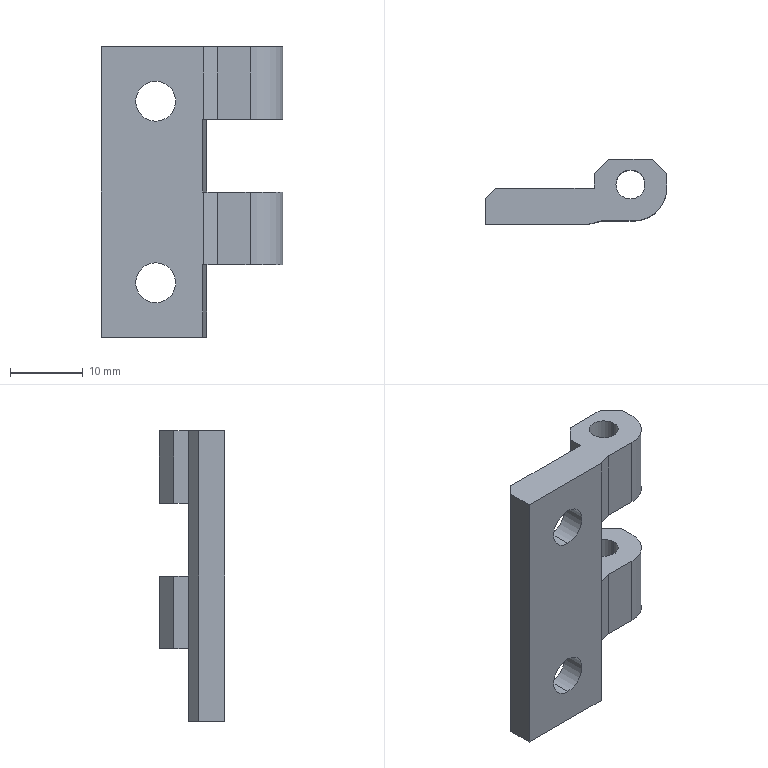Part | SolidWorks | features BaseBody 1 | 1 solid | 41 faces | box 25 x 9 x 40 mm | volume 3717 mm3 | plane 27 | cylinder 14 | commonest cylinder face diameters 4 x4 5.5 x4 10.5 x4 9 x2
STEP:
#1=CARTESIAN_POINT('',(-12.5,3.3,15.25));
#2=VERTEX_POINT('',#1);
#3=CARTESIAN_POINT('',(-12.5,3.3,9.75));
#4=VERTEX_POINT('',#3);
#5=CARTESIAN_POINT('',(-12.5,3.3,12.5));
#6=DIRECTION('',(0.,-1.,0.));
#7=DIRECTION('',(0.,0.,-1.));
#8=AXIS2_PLACEMENT_3D('',#5,#6,#7);
#9=CIRCLE('',#8,2.75);
#10=EDGE_CURVE('',#2,#4,#9,.T.);
#11=ORIENTED_EDGE('',*,*,#10,.F.);
#12=CARTESIAN_POINT('',(-12.5,0.,15.25));
#13=VERTEX_POINT('',#12);
#14=CARTESIAN_POINT('',(-12.5,0.,15.25));
#15=DIRECTION('',(0.,-1.,0.));
#16=VECTOR('',#15,1000.);
#17=LINE('',#14,#16);
#18=EDGE_CURVE('',#2,#13,#17,.T.);
#19=ORIENTED_EDGE('',*,*,#18,.T.);
#20=CARTESIAN_POINT('',(-12.5,0.,9.75));
#21=VERTEX_POINT('',#20);
#22=CARTESIAN_POINT('',(-12.5,0.,12.5));
#23=DIRECTION('',(0.,-1.,0.));
#24=DIRECTION('',(0.,0.,-1.));
#25=AXIS2_PLACEMENT_3D('',#22,#23,#24);
#26=CIRCLE('',#25,2.75);
#27=EDGE_CURVE('',#13,#21,#26,.T.);
#28=ORIENTED_EDGE('',*,*,#27,.T.);
#29=CARTESIAN_POINT('',(-12.5,0.,9.75));
#30=DIRECTION('',(0.,-1.,0.));
#31=VECTOR('',#30,1000.);
#32=LINE('',#29,#31);
#33=EDGE_CURVE('',#4,#21,#32,.T.);
#34=ORIENTED_EDGE('',*,*,#33,.F.);
#35=EDGE_LOOP('',(#11,#19,#28,#34));
#36=FACE_OUTER_BOUND('',#35,.T.);
#37=CARTESIAN_POINT('',(-12.5,0.,12.5));
#38=DIRECTION('',(0.,-1.,0.));
#39=DIRECTION('',(0.,0.,-1.));
#40=AXIS2_PLACEMENT_3D('',#37,#38,#39);
#41=CYLINDRICAL_SURFACE('',#40,2.75);
#42=ADVANCED_FACE('',(#36),#41,.F.);
#43=CARTESIAN_POINT('',(-12.5,3.3,-9.75));
#44=VERTEX_POINT('',#43);
#45=CARTESIAN_POINT('',(-12.5,3.3,-15.25));
#46=VERTEX_POINT('',#45);
#47=CARTESIAN_POINT('',(-12.5,3.3,-12.5));
#48=DIRECTION('',(0.,-1.,0.));
#49=DIRECTION('',(0.,0.,-1.));
#50=AXIS2_PLACEMENT_3D('',#47,#48,#49);
#51=CIRCLE('',#50,2.75);
#52=EDGE_CURVE('',#44,#46,#51,.T.);
#53=ORIENTED_EDGE('',*,*,#52,.F.);
#54=CARTESIAN_POINT('',(-12.5,0.,-9.75));
#55=VERTEX_POINT('',#54);
#56=CARTESIAN_POINT('',(-12.5,0.,-9.75));
#57=DIRECTION('',(0.,-1.,0.));
#58=VECTOR('',#57,1000.);
#59=LINE('',#56,#58);
#60=EDGE_CURVE('',#44,#55,#59,.T.);
#61=ORIENTED_EDGE('',*,*,#60,.T.);
#62=CARTESIAN_POINT('',(-12.5,0.,-15.25));
#63=VERTEX_POINT('',#62);
#64=CARTESIAN_POINT('',(-12.5,0.,-12.5));
#65=DIRECTION('',(0.,-1.,0.));
#66=DIRECTION('',(0.,0.,-1.));
#67=AXIS2_PLACEMENT_3D('',#64,#65,#66);
#68=CIRCLE('',#67,2.75);
#69=EDGE_CURVE('',#55,#63,#68,.T.);
#70=ORIENTED_EDGE('',*,*,#69,.T.);
#71=CARTESIAN_POINT('',(-12.5,0.,-15.25));
#72=DIRECTION('',(0.,-1.,0.));
#73=VECTOR('',#72,1000.);
#74=LINE('',#71,#73);
#75=EDGE_CURVE('',#46,#63,#74,.T.);
#76=ORIENTED_EDGE('',*,*,#75,.F.);
#77=EDGE_LOOP('',(#53,#61,#70,#76));
#78=FACE_OUTER_BOUND('',#77,.T.);
#79=CARTESIAN_POINT('',(-12.5,0.,-12.5));
#80=DIRECTION('',(0.,-1.,0.));
#81=DIRECTION('',(0.,0.,-1.));
#82=AXIS2_PLACEMENT_3D('',#79,#80,#81);
#83=CYLINDRICAL_SURFACE('',#82,2.75);
#84=ADVANCED_FACE('',(#78),#83,.F.);
#85=CARTESIAN_POINT('',(2.,5.5,20.));
#86=VERTEX_POINT('',#85);
#87=CARTESIAN_POINT('',(-2.,5.5,20.));
#88=VERTEX_POINT('',#87);
#89=CARTESIAN_POINT('',(0.,5.5,20.));
#90=DIRECTION('',(0.,0.,-1.));
#91=DIRECTION('',(-1.,0.,0.));
#92=AXIS2_PLACEMENT_3D('',#89,#90,#91);
#93=CIRCLE('',#92,2.);
#94=EDGE_CURVE('',#86,#88,#93,.T.);
#95=ORIENTED_EDGE('',*,*,#94,.F.);
#96=CARTESIAN_POINT('',(2.,5.5,10.));
#97=VERTEX_POINT('',#96);
#98=CARTESIAN_POINT('',(2.,5.5,20.));
#99=DIRECTION('',(0.,0.,-1.));
#100=VECTOR('',#99,1000.);
#101=LINE('',#98,#100);
#102=EDGE_CURVE('',#86,#97,#101,.T.);
#103=ORIENTED_EDGE('',*,*,#102,.T.);
#104=CARTESIAN_POINT('',(-2.,5.5,10.));
#105=VERTEX_POINT('',#104);
#106=CARTESIAN_POINT('',(0.,5.5,10.));
#107=DIRECTION('',(0.,0.,-1.));
#108=DIRECTION('',(-1.,0.,0.));
#109=AXIS2_PLACEMENT_3D('',#106,#107,#108);
#110=CIRCLE('',#109,2.);
#111=EDGE_CURVE('',#97,#105,#110,.T.);
#112=ORIENTED_EDGE('',*,*,#111,.T.);
#113=CARTESIAN_POINT('',(-2.,5.5,20.));
#114=DIRECTION('',(0.,0.,-1.));
#115=VECTOR('',#114,1000.);
#116=LINE('',#113,#115);
#117=EDGE_CURVE('',#88,#105,#116,.T.);
#118=ORIENTED_EDGE('',*,*,#117,.F.);
#119=EDGE_LOOP('',(#95,#103,#112,#118));
#120=FACE_OUTER_BOUND('',#119,.T.);
#121=CARTESIAN_POINT('',(0.,5.5,20.));
#122=DIRECTION('',(0.,0.,-1.));
#123=DIRECTION('',(-1.,0.,0.));
#124=AXIS2_PLACEMENT_3D('',#121,#122,#123);
#125=CYLINDRICAL_SURFACE('',#124,2.);
#126=ADVANCED_FACE('',(#120),#125,.F.);
#127=CARTESIAN_POINT('',(-12.5,5.,7.25));
#128=VERTEX_POINT('',#127);
#129=CARTESIAN_POINT('',(-12.5,5.,17.75));
#130=VERTEX_POINT('',#129);
#131=CARTESIAN_POINT('',(-12.5,5.,12.5));
#132=DIRECTION('',(0.,1.,0.));
#133=DIRECTION('',(0.,0.,-1.));
#134=AXIS2_PLACEMENT_3D('',#131,#132,#133);
#135=CIRCLE('',#134,5.25);
#136=EDGE_CURVE('',#128,#130,#135,.T.);
#137=ORIENTED_EDGE('',*,*,#136,.T.);
#138=CARTESIAN_POINT('',(-12.5,3.3,17.75));
#139=VERTEX_POINT('',#138);
#140=CARTESIAN_POINT('',(-12.5,0.,17.75));
#141=DIRECTION('',(0.,-1.,0.));
#142=VECTOR('',#141,1000.);
#143=LINE('',#140,#142);
#144=EDGE_CURVE('',#130,#139,#143,.T.);
#145=ORIENTED_EDGE('',*,*,#144,.T.);
#146=CARTESIAN_POINT('',(-12.5,3.3,7.25));
#147=VERTEX_POINT('',#146);
#148=CARTESIAN_POINT('',(-12.5,3.3,12.5));
#149=DIRECTION('',(0.,1.,0.));
#150=DIRECTION('',(0.,0.,-1.));
#151=AXIS2_PLACEMENT_3D('',#148,#149,#150);
#152=CIRCLE('',#151,5.25);
#153=EDGE_CURVE('',#147,#139,#152,.T.);
#154=ORIENTED_EDGE('',*,*,#153,.F.);
#155=CARTESIAN_POINT('',(-12.5,0.,7.25));
#156=DIRECTION('',(0.,-1.,0.));
#157=VECTOR('',#156,1000.);
#158=LINE('',#155,#157);
#159=EDGE_CURVE('',#128,#147,#158,.T.);
#160=ORIENTED_EDGE('',*,*,#159,.F.);
#161=EDGE_LOOP('',(#137,#145,#154,#160));
#162=FACE_OUTER_BOUND('',#161,.T.);
#163=CARTESIAN_POINT('',(-12.5,0.,12.5));
#164=DIRECTION('',(0.,-1.,0.));
#165=DIRECTION('',(0.,0.,-1.));
#166=AXIS2_PLACEMENT_3D('',#163,#164,#165);
#167=CYLINDRICAL_SURFACE('',#166,5.25);
#168=ADVANCED_FACE('',(#162),#167,.F.);
#169=CARTESIAN_POINT('',(-12.5,5.,-17.75));
#170=VERTEX_POINT('',#169);
#171=CARTESIAN_POINT('',(-12.5,5.,-7.25));
#172=VERTEX_POINT('',#171);
#173=CARTESIAN_POINT('',(-12.5,5.,-12.5));
#174=DIRECTION('',(0.,1.,0.));
#175=DIRECTION('',(0.,0.,-1.));
#176=AXIS2_PLACEMENT_3D('',#173,#174,#175);
#177=CIRCLE('',#176,5.25);
#178=EDGE_CURVE('',#170,#172,#177,.T.);
#179=ORIENTED_EDGE('',*,*,#178,.T.);
#180=CARTESIAN_POINT('',(-12.5,3.3,-7.25));
#181=VERTEX_POINT('',#180);
#182=CARTESIAN_POINT('',(-12.5,0.,-7.25));
#183=DIRECTION('',(0.,-1.,0.));
#184=VECTOR('',#183,1000.);
#185=LINE('',#182,#184);
#186=EDGE_CURVE('',#172,#181,#185,.T.);
#187=ORIENTED_EDGE('',*,*,#186,.T.);
#188=CARTESIAN_POINT('',(-12.5,3.3,-17.75));
#189=VERTEX_POINT('',#188);
#190=CARTESIAN_POINT('',(-12.5,3.3,-12.5));
#191=DIRECTION('',(0.,1.,0.));
#192=DIRECTION('',(0.,0.,-1.));
#193=AXIS2_PLACEMENT_3D('',#190,#191,#192);
#194=CIRCLE('',#193,5.25);
#195=EDGE_CURVE('',#189,#181,#194,.T.);
#196=ORIENTED_EDGE('',*,*,#195,.F.);
#197=CARTESIAN_POINT('',(-12.5,0.,-17.75));
#198=DIRECTION('',(0.,-1.,0.));
#199=VECTOR('',#198,1000.);
#200=LINE('',#197,#199);
#201=EDGE_CURVE('',#170,#189,#200,.T.);
#202=ORIENTED_EDGE('',*,*,#201,.F.);
#203=EDGE_LOOP('',(#179,#187,#196,#202));
#204=FACE_OUTER_BOUND('',#203,.T.);
#205=CARTESIAN_POINT('',(-12.5,0.,-12.5));
#206=DIRECTION('',(0.,-1.,0.));
#207=DIRECTION('',(0.,0.,-1.));
#208=AXIS2_PLACEMENT_3D('',#205,#206,#207);
#209=CYLINDRICAL_SURFACE('',#208,5.25);
#210=ADVANCED_FACE('',(#204),#209,.F.);
#211=CARTESIAN_POINT('',(2.,5.5,-10.));
#212=VERTEX_POINT('',#211);
#213=CARTESIAN_POINT('',(-2.,5.5,-10.));
#214=VERTEX_POINT('',#213);
#215=CARTESIAN_POINT('',(0.,5.5,-10.));
#216=DIRECTION('',(0.,0.,-1.));
#217=DIRECTION('',(1.,0.,0.));
#218=AXIS2_PLACEMENT_3D('',#215,#216,#217);
#219=CIRCLE('',#218,2.);
#220=EDGE_CURVE('',#212,#214,#219,.T.);
#221=ORIENTED_EDGE('',*,*,#220,.T.);
#222=CARTESIAN_POINT('',(-2.,5.5,0.));
#223=VERTEX_POINT('',#222);
#224=CARTESIAN_POINT('',(-2.,5.5,-10.));
#225=DIRECTION('',(0.,0.,1.));
#226=VECTOR('',#225,1000.);
#227=LINE('',#224,#226);
#228=EDGE_CURVE('',#214,#223,#227,.T.);
#229=ORIENTED_EDGE('',*,*,#228,.T.);
#230=CARTESIAN_POINT('',(2.,5.5,0.));
#231=VERTEX_POINT('',#230);
#232=CARTESIAN_POINT('',(0.,5.5,0.));
#233=DIRECTION('',(0.,0.,-1.));
#234=DIRECTION('',(1.,0.,0.));
#235=AXIS2_PLACEMENT_3D('',#232,#233,#234);
#236=CIRCLE('',#235,2.);
#237=EDGE_CURVE('',#231,#223,#236,.T.);
#238=ORIENTED_EDGE('',*,*,#237,.F.);
#239=CARTESIAN_POINT('',(2.,5.5,-10.));
#240=DIRECTION('',(0.,0.,1.));
#241=VECTOR('',#240,1000.);
#242=LINE('',#239,#241);
#243=EDGE_CURVE('',#212,#231,#242,.T.);
#244=ORIENTED_EDGE('',*,*,#243,.F.);
#245=EDGE_LOOP('',(#221,#229,#238,#244));
#246=FACE_OUTER_BOUND('',#245,.T.);
#247=CARTESIAN_POINT('',(0.,5.5,-10.));
#248=DIRECTION('',(0.,0.,1.));
#249=DIRECTION('',(1.,0.,0.));
#250=AXIS2_PLACEMENT_3D('',#247,#248,#249);
#251=CYLINDRICAL_SURFACE('',#250,2.);
#252=ADVANCED_FACE('',(#246),#251,.F.);
#253=CARTESIAN_POINT('',(-20.,0.,20.));
#254=VERTEX_POINT('',#253);
#255=CARTESIAN_POINT('',(-5.866,0.,20.));
#256=VERTEX_POINT('',#255);
#257=CARTESIAN_POINT('',(-20.,0.,20.));
#258=DIRECTION('',(1.,0.,0.));
#259=VECTOR('',#258,1000.);
#260=LINE('',#257,#259);
#261=EDGE_CURVE('',#254,#256,#260,.T.);
#262=ORIENTED_EDGE('',*,*,#261,.F.);
#263=CARTESIAN_POINT('',(-20.,0.,-20.));
#264=VERTEX_POINT('',#263);
#265=CARTESIAN_POINT('',(-20.,0.,20.));
#266=DIRECTION('',(0.,0.,1.));
#267=VECTOR('',#266,1000.);
#268=LINE('',#265,#267);
#269=EDGE_CURVE('',#264,#254,#268,.T.);
#270=ORIENTED_EDGE('',*,*,#269,.F.);
#271=CARTESIAN_POINT('',(-6.,0.,-20.));
#272=VERTEX_POINT('',#271);
#273=CARTESIAN_POINT('',(-20.,0.,-20.));
#274=DIRECTION('',(-1.,0.,0.));
#275=VECTOR('',#274,1000.);
#276=LINE('',#273,#275);
#277=EDGE_CURVE('',#272,#264,#276,.T.);
#278=ORIENTED_EDGE('',*,*,#277,.F.);
#279=CARTESIAN_POINT('',(-6.,0.,-10.));
#280=VERTEX_POINT('',#279);
#281=CARTESIAN_POINT('',(-6.,0.,20.));
#282=DIRECTION('',(0.,0.,-1.));
#283=VECTOR('',#282,1000.);
#284=LINE('',#281,#283);
#285=EDGE_CURVE('',#280,#272,#284,.T.);
#286=ORIENTED_EDGE('',*,*,#285,.F.);
#287=CARTESIAN_POINT('',(-5.866,0.,-10.));
#288=VERTEX_POINT('',#287);
#289=CARTESIAN_POINT('',(0.5,0.,-10.));
#290=DIRECTION('',(1.,0.,0.));
#291=VECTOR('',#290,1000.);
#292=LINE('',#289,#291);
#293=EDGE_CURVE('',#280,#288,#292,.T.);
#294=ORIENTED_EDGE('',*,*,#293,.T.);
#295=CARTESIAN_POINT('',(-5.866,0.,0.));
#296=VERTEX_POINT('',#295);
#297=CARTESIAN_POINT('',(-5.866,0.,20.));
#298=DIRECTION('',(0.,0.,-1.));
#299=VECTOR('',#298,1000.);
#300=LINE('',#297,#299);
#301=EDGE_CURVE('',#296,#288,#300,.T.);
#302=ORIENTED_EDGE('',*,*,#301,.F.);
#303=CARTESIAN_POINT('',(-6.,0.,0.));
#304=VERTEX_POINT('',#303);
#305=CARTESIAN_POINT('',(0.5,0.,0.));
#306=DIRECTION('',(1.,0.,0.));
#307=VECTOR('',#306,1000.);
#308=LINE('',#305,#307);
#309=EDGE_CURVE('',#304,#296,#308,.T.);
#310=ORIENTED_EDGE('',*,*,#309,.F.);
#311=CARTESIAN_POINT('',(-6.,0.,10.));
#312=VERTEX_POINT('',#311);
#313=CARTESIAN_POINT('',(-6.,0.,20.));
#314=DIRECTION('',(0.,0.,-1.));
#315=VECTOR('',#314,1000.);
#316=LINE('',#313,#315);
#317=EDGE_CURVE('',#312,#304,#316,.T.);
#318=ORIENTED_EDGE('',*,*,#317,.F.);
#319=CARTESIAN_POINT('',(-5.866,0.,10.));
#320=VERTEX_POINT('',#319);
#321=CARTESIAN_POINT('',(0.5,0.,10.));
#322=DIRECTION('',(1.,0.,0.));
#323=VECTOR('',#322,1000.);
#324=LINE('',#321,#323);
#325=EDGE_CURVE('',#312,#320,#324,.T.);
#326=ORIENTED_EDGE('',*,*,#325,.T.);
#327=CARTESIAN_POINT('',(-5.866,0.,20.));
#328=DIRECTION('',(0.,0.,-1.));
#329=VECTOR('',#328,1000.);
#330=LINE('',#327,#329);
#331=EDGE_CURVE('',#256,#320,#330,.T.);
#332=ORIENTED_EDGE('',*,*,#331,.F.);
#333=EDGE_LOOP('',(#262,#270,#278,#286,#294,#302,#310,#318,#326,#332));
#334=FACE_OUTER_BOUND('',#333,.T.);
#335=CARTESIAN_POINT('',(-12.5,0.,12.5));
#336=DIRECTION('',(0.,-1.,0.));
#337=DIRECTION('',(0.,0.,-1.));
#338=AXIS2_PLACEMENT_3D('',#335,#336,#337);
#339=CIRCLE('',#338,2.75);
#340=EDGE_CURVE('',#21,#13,#339,.T.);
#341=ORIENTED_EDGE('',*,*,#340,.F.);
#342=ORIENTED_EDGE('',*,*,#27,.F.);
#343=EDGE_LOOP('',(#341,#342));
#344=FACE_BOUND('',#343,.T.);
#345=CARTESIAN_POINT('',(-12.5,0.,-12.5));
#346=DIRECTION('',(0.,-1.,0.));
#347=DIRECTION('',(0.,0.,-1.));
#348=AXIS2_PLACEMENT_3D('',#345,#346,#347);
#349=CIRCLE('',#348,2.75);
#350=EDGE_CURVE('',#63,#55,#349,.T.);
#351=ORIENTED_EDGE('',*,*,#350,.F.);
#352=ORIENTED_EDGE('',*,*,#69,.F.);
#353=EDGE_LOOP('',(#351,#352));
#354=FACE_BOUND('',#353,.T.);
#355=CARTESIAN_POINT('',(-20.,0.,20.));
#356=DIRECTION('',(0.,1.,0.));
#357=DIRECTION('',(0.,0.,1.));
#358=AXIS2_PLACEMENT_3D('',#355,#356,#357);
#359=PLANE('',#358);
#360=ADVANCED_FACE('',(#334,#344,#354),#359,.F.);
#361=CARTESIAN_POINT('',(-4.,0.5,20.));
#362=VERTEX_POINT('',#361);
#363=CARTESIAN_POINT('',(-4.,0.5,10.));
#364=VERTEX_POINT('',#363);
#365=CARTESIAN_POINT('',(-4.,0.5,20.));
#366=DIRECTION('',(0.,0.,-1.));
#367=VECTOR('',#366,1000.);
#368=LINE('',#365,#367);
#369=EDGE_CURVE('',#362,#364,#368,.T.);
#370=ORIENTED_EDGE('',*,*,#369,.F.);
#371=CARTESIAN_POINT('',(-5.866,0.,20.));
#372=DIRECTION('',(0.9659,0.2588,0.));
#373=VECTOR('',#372,1000.);
#374=LINE('',#371,#373);
#375=EDGE_CURVE('',#256,#362,#374,.T.);
#376=ORIENTED_EDGE('',*,*,#375,.F.);
#377=ORIENTED_EDGE('',*,*,#331,.T.);
#378=CARTESIAN_POINT('',(-5.866,0.,10.));
#379=DIRECTION('',(-0.9659,-0.2588,0.));
#380=VECTOR('',#379,1000.);
#381=LINE('',#378,#380);
#382=EDGE_CURVE('',#364,#320,#381,.T.);
#383=ORIENTED_EDGE('',*,*,#382,.F.);
#384=EDGE_LOOP('',(#370,#376,#377,#383));
#385=FACE_OUTER_BOUND('',#384,.T.);
#386=CARTESIAN_POINT('',(-5.866,0.,20.));
#387=DIRECTION('',(-0.2588,0.9659,0.));
#388=DIRECTION('',(-0.9659,-0.2588,0.));
#389=AXIS2_PLACEMENT_3D('',#386,#387,#388);
#390=PLANE('',#389);
#391=ADVANCED_FACE('',(#385),#390,.F.);
#392=CARTESIAN_POINT('',(0.,5.5,20.));
#393=DIRECTION('',(0.,0.,-1.));
#394=DIRECTION('',(-1.,0.,0.));
#395=AXIS2_PLACEMENT_3D('',#392,#393,#394);
#396=CIRCLE('',#395,2.);
#397=EDGE_CURVE('',#88,#86,#396,.T.);
#398=ORIENTED_EDGE('',*,*,#397,.T.);
#399=ORIENTED_EDGE('',*,*,#94,.T.);
#400=EDGE_LOOP('',(#398,#399));
#401=FACE_BOUND('',#400,.T.);
#402=CARTESIAN_POINT('',(-3.,9.,20.));
#403=VERTEX_POINT('',#402);
#404=CARTESIAN_POINT('',(-5.,7.,20.));
#405=VERTEX_POINT('',#404);
#406=CARTESIAN_POINT('',(-3.,9.,20.));
#407=DIRECTION('',(-0.7071,-0.7071,0.));
#408=VECTOR('',#407,1000.);
#409=LINE('',#406,#408);
#410=EDGE_CURVE('',#403,#405,#409,.T.);
#411=ORIENTED_EDGE('',*,*,#410,.T.);
#412=CARTESIAN_POINT('',(-5.,5.,20.));
#413=VERTEX_POINT('',#412);
#414=CARTESIAN_POINT('',(-5.,0.,20.));
#415=DIRECTION('',(0.,-1.,0.));
#416=VECTOR('',#415,1000.);
#417=LINE('',#414,#416);
#418=EDGE_CURVE('',#405,#413,#417,.T.);
#419=ORIENTED_EDGE('',*,*,#418,.T.);
#420=CARTESIAN_POINT('',(-18.6,5.,20.));
#421=VERTEX_POINT('',#420);
#422=CARTESIAN_POINT('',(0.,5.,20.));
#423=DIRECTION('',(-1.,0.,0.));
#424=VECTOR('',#423,1000.);
#425=LINE('',#422,#424);
#426=EDGE_CURVE('',#413,#421,#425,.T.);
#427=ORIENTED_EDGE('',*,*,#426,.T.);
#428=CARTESIAN_POINT('',(-20.,3.6,20.));
#429=VERTEX_POINT('',#428);
#430=CARTESIAN_POINT('',(-18.6,5.,20.));
#431=DIRECTION('',(-0.7071,-0.7071,0.));
#432=VECTOR('',#431,1000.);
#433=LINE('',#430,#432);
#434=EDGE_CURVE('',#421,#429,#433,.T.);
#435=ORIENTED_EDGE('',*,*,#434,.T.);
#436=CARTESIAN_POINT('',(-20.,0.,20.));
#437=DIRECTION('',(0.,-1.,0.));
#438=VECTOR('',#437,1000.);
#439=LINE('',#436,#438);
#440=EDGE_CURVE('',#429,#254,#439,.T.);
#441=ORIENTED_EDGE('',*,*,#440,.T.);
#442=ORIENTED_EDGE('',*,*,#261,.T.);
#443=ORIENTED_EDGE('',*,*,#375,.T.);
#444=CARTESIAN_POINT('',(0.5,0.5,20.));
#445=VERTEX_POINT('',#444);
#446=CARTESIAN_POINT('',(0.,0.5,20.));
#447=DIRECTION('',(1.,0.,0.));
#448=VECTOR('',#447,1000.);
#449=LINE('',#446,#448);
#450=EDGE_CURVE('',#362,#445,#449,.T.);
#451=ORIENTED_EDGE('',*,*,#450,.T.);
#452=CARTESIAN_POINT('',(5.,5.,20.));
#453=VERTEX_POINT('',#452);
#454=CARTESIAN_POINT('',(0.5,5.,20.));
#455=DIRECTION('',(0.,0.,1.));
#456=DIRECTION('',(-1.,0.,0.));
#457=AXIS2_PLACEMENT_3D('',#454,#455,#456);
#458=CIRCLE('',#457,4.5);
#459=EDGE_CURVE('',#445,#453,#458,.T.);
#460=ORIENTED_EDGE('',*,*,#459,.T.);
#461=CARTESIAN_POINT('',(5.,7.,20.));
#462=VERTEX_POINT('',#461);
#463=CARTESIAN_POINT('',(5.,0.,20.));
#464=DIRECTION('',(0.,1.,0.));
#465=VECTOR('',#464,1000.);
#466=LINE('',#463,#465);
#467=EDGE_CURVE('',#453,#462,#466,.T.);
#468=ORIENTED_EDGE('',*,*,#467,.T.);
#469=CARTESIAN_POINT('',(3.,9.,20.));
#470=VERTEX_POINT('',#469);
#471=CARTESIAN_POINT('',(5.,7.,20.));
#472=DIRECTION('',(-0.7071,0.7071,0.));
#473=VECTOR('',#472,1000.);
#474=LINE('',#471,#473);
#475=EDGE_CURVE('',#462,#470,#474,.T.);
#476=ORIENTED_EDGE('',*,*,#475,.T.);
#477=CARTESIAN_POINT('',(0.,9.,20.));
#478=DIRECTION('',(-1.,0.,0.));
#479=VECTOR('',#478,1000.);
#480=LINE('',#477,#479);
#481=EDGE_CURVE('',#470,#403,#480,.T.);
#482=ORIENTED_EDGE('',*,*,#481,.T.);
#483=EDGE_LOOP('',(#411,#419,#427,#435,#441,#442,#443,#451,#460,#468,#476,#482));
#484=FACE_OUTER_BOUND('',#483,.T.);
#485=CARTESIAN_POINT('',(0.,0.,20.));
#486=DIRECTION('',(0.,0.,1.));
#487=DIRECTION('',(1.,0.,0.));
#488=AXIS2_PLACEMENT_3D('',#485,#486,#487);
#489=PLANE('',#488);
#490=ADVANCED_FACE('',(#401,#484),#489,.T.);
#491=ORIENTED_EDGE('',*,*,#269,.T.);
#492=ORIENTED_EDGE('',*,*,#440,.F.);
#493=CARTESIAN_POINT('',(-20.,3.6,-20.));
#494=VERTEX_POINT('',#493);
#495=CARTESIAN_POINT('',(-20.,3.6,20.));
#496=DIRECTION('',(0.,0.,1.));
#497=VECTOR('',#496,1000.);
#498=LINE('',#495,#497);
#499=EDGE_CURVE('',#494,#429,#498,.T.);
#500=ORIENTED_EDGE('',*,*,#499,.F.);
#501=CARTESIAN_POINT('',(-20.,3.6,-20.));
#502=DIRECTION('',(0.,1.,0.));
#503=VECTOR('',#502,1000.);
#504=LINE('',#501,#503);
#505=EDGE_CURVE('',#264,#494,#504,.T.);
#506=ORIENTED_EDGE('',*,*,#505,.F.);
#507=EDGE_LOOP('',(#491,#492,#500,#506));
#508=FACE_OUTER_BOUND('',#507,.T.);
#509=CARTESIAN_POINT('',(-20.,3.6,20.));
#510=DIRECTION('',(1.,0.,0.));
#511=DIRECTION('',(0.,0.,-1.));
#512=AXIS2_PLACEMENT_3D('',#509,#510,#511);
#513=PLANE('',#512);
#514=ADVANCED_FACE('',(#508),#513,.F.);
#515=CARTESIAN_POINT('',(-5.5,5.,-20.));
#516=VERTEX_POINT('',#515);
#517=CARTESIAN_POINT('',(-18.6,5.,-20.));
#518=VERTEX_POINT('',#517);
#519=CARTESIAN_POINT('',(0.,5.,-20.));
#520=DIRECTION('',(-1.,0.,0.));
#521=VECTOR('',#520,1000.);
#522=LINE('',#519,#521);
#523=EDGE_CURVE('',#516,#518,#522,.T.);
#524=ORIENTED_EDGE('',*,*,#523,.F.);
#525=CARTESIAN_POINT('',(-6.,0.,-20.));
#526=DIRECTION('',(0.0995,0.995,0.));
#527=VECTOR('',#526,1000.);
#528=LINE('',#525,#527);
#529=EDGE_CURVE('',#272,#516,#528,.T.);
#530=ORIENTED_EDGE('',*,*,#529,.F.);
#531=ORIENTED_EDGE('',*,*,#277,.T.);
#532=ORIENTED_EDGE('',*,*,#505,.T.);
#533=CARTESIAN_POINT('',(-18.6,5.,-20.));
#534=DIRECTION('',(-0.7071,-0.7071,0.));
#535=VECTOR('',#534,1000.);
#536=LINE('',#533,#535);
#537=EDGE_CURVE('',#518,#494,#536,.T.);
#538=ORIENTED_EDGE('',*,*,#537,.F.);
#539=EDGE_LOOP('',(#524,#530,#531,#532,#538));
#540=FACE_OUTER_BOUND('',#539,.T.);
#541=CARTESIAN_POINT('',(0.,0.,-20.));
#542=DIRECTION('',(0.,0.,1.));
#543=DIRECTION('',(1.,0.,0.));
#544=AXIS2_PLACEMENT_3D('',#541,#542,#543);
#545=PLANE('',#544);
#546=ADVANCED_FACE('',(#540),#545,.F.);
#547=ORIENTED_EDGE('',*,*,#285,.T.);
#548=ORIENTED_EDGE('',*,*,#529,.T.);
#549=CARTESIAN_POINT('',(-5.5,5.,-10.));
#550=VERTEX_POINT('',#549);
#551=CARTESIAN_POINT('',(-5.5,5.,20.));
#552=DIRECTION('',(0.,0.,-1.));
#553=VECTOR('',#552,1000.);
#554=LINE('',#551,#553);
#555=EDGE_CURVE('',#550,#516,#554,.T.);
#556=ORIENTED_EDGE('',*,*,#555,.F.);
#557=CARTESIAN_POINT('',(-6.,0.,-10.));
#558=DIRECTION('',(0.0995,0.995,0.));
#559=VECTOR('',#558,1000.);
#560=LINE('',#557,#559);
#561=EDGE_CURVE('',#280,#550,#560,.T.);
#562=ORIENTED_EDGE('',*,*,#561,.F.);
#563=EDGE_LOOP('',(#547,#548,#556,#562));
#564=FACE_OUTER_BOUND('',#563,.T.);
#565=CARTESIAN_POINT('',(-6.,0.,20.));
#566=DIRECTION('',(-0.995,0.0995,0.));
#567=DIRECTION('',(-0.0995,-0.995,0.));
#568=AXIS2_PLACEMENT_3D('',#565,#566,#567);
#569=PLANE('',#568);
#570=ADVANCED_FACE('',(#564),#569,.F.);
#571=CARTESIAN_POINT('',(-4.,0.5,-10.));
#572=VERTEX_POINT('',#571);
#573=CARTESIAN_POINT('',(-5.866,0.,-10.));
#574=DIRECTION('',(0.9659,0.2588,0.));
#575=VECTOR('',#574,1000.);
#576=LINE('',#573,#575);
#577=EDGE_CURVE('',#288,#572,#576,.T.);
#578=ORIENTED_EDGE('',*,*,#577,.T.);
#579=CARTESIAN_POINT('',(-4.,0.5,0.));
#580=VERTEX_POINT('',#579);
#581=CARTESIAN_POINT('',(-4.,0.5,-10.));
#582=DIRECTION('',(0.,0.,1.));
#583=VECTOR('',#582,1000.);
#584=LINE('',#581,#583);
#585=EDGE_CURVE('',#572,#580,#584,.T.);
#586=ORIENTED_EDGE('',*,*,#585,.T.);
#587=CARTESIAN_POINT('',(-5.866,0.,0.));
#588=DIRECTION('',(-0.9659,-0.2588,0.));
#589=VECTOR('',#588,1000.);
#590=LINE('',#587,#589);
#591=EDGE_CURVE('',#580,#296,#590,.T.);
#592=ORIENTED_EDGE('',*,*,#591,.T.);
#593=ORIENTED_EDGE('',*,*,#301,.T.);
#594=EDGE_LOOP('',(#578,#586,#592,#593));
#595=FACE_OUTER_BOUND('',#594,.T.);
#596=CARTESIAN_POINT('',(-5.866,0.,-10.));
#597=DIRECTION('',(0.2588,-0.9659,0.));
#598=DIRECTION('',(0.9659,0.2588,0.));
#599=AXIS2_PLACEMENT_3D('',#596,#597,#598);
#600=PLANE('',#599);
#601=ADVANCED_FACE('',(#595),#600,.T.);
#602=ORIENTED_EDGE('',*,*,#317,.T.);
#603=CARTESIAN_POINT('',(-5.5,5.,0.));
#604=VERTEX_POINT('',#603);
#605=CARTESIAN_POINT('',(-6.,0.,0.));
#606=DIRECTION('',(-0.0995,-0.995,0.));
#607=VECTOR('',#606,1000.);
#608=LINE('',#605,#607);
#609=EDGE_CURVE('',#604,#304,#608,.T.);
#610=ORIENTED_EDGE('',*,*,#609,.F.);
#611=CARTESIAN_POINT('',(-5.5,5.,10.));
#612=VERTEX_POINT('',#611);
#613=CARTESIAN_POINT('',(-5.5,5.,20.));
#614=DIRECTION('',(0.,0.,-1.));
#615=VECTOR('',#614,1000.);
#616=LINE('',#613,#615);
#617=EDGE_CURVE('',#612,#604,#616,.T.);
#618=ORIENTED_EDGE('',*,*,#617,.F.);
#619=CARTESIAN_POINT('',(-6.,0.,10.));
#620=DIRECTION('',(0.0995,0.995,0.));
#621=VECTOR('',#620,1000.);
#622=LINE('',#619,#621);
#623=EDGE_CURVE('',#312,#612,#622,.T.);
#624=ORIENTED_EDGE('',*,*,#623,.F.);
#625=EDGE_LOOP('',(#602,#610,#618,#624));
#626=FACE_OUTER_BOUND('',#625,.T.);
#627=CARTESIAN_POINT('',(-6.,0.,20.));
#628=DIRECTION('',(-0.995,0.0995,0.));
#629=DIRECTION('',(-0.0995,-0.995,0.));
#630=AXIS2_PLACEMENT_3D('',#627,#628,#629);
#631=PLANE('',#630);
#632=ADVANCED_FACE('',(#626),#631,.F.);
#633=ORIENTED_EDGE('',*,*,#18,.F.);
#634=CARTESIAN_POINT('',(-12.5,3.3,12.5));
#635=DIRECTION('',(0.,-1.,0.));
#636=DIRECTION('',(0.,0.,-1.));
#637=AXIS2_PLACEMENT_3D('',#634,#635,#636);
#638=CIRCLE('',#637,2.75);
#639=EDGE_CURVE('',#4,#2,#638,.T.);
#640=ORIENTED_EDGE('',*,*,#639,.F.);
#641=ORIENTED_EDGE('',*,*,#33,.T.);
#642=ORIENTED_EDGE('',*,*,#340,.T.);
#643=EDGE_LOOP('',(#633,#640,#641,#642));
#644=FACE_OUTER_BOUND('',#643,.T.);
#645=CARTESIAN_POINT('',(-12.5,0.,12.5));
#646=DIRECTION('',(0.,-1.,0.));
#647=DIRECTION('',(0.,0.,-1.));
#648=AXIS2_PLACEMENT_3D('',#645,#646,#647);
#649=CYLINDRICAL_SURFACE('',#648,2.75);
#650=ADVANCED_FACE('',(#644),#649,.F.);
#651=ORIENTED_EDGE('',*,*,#60,.F.);
#652=CARTESIAN_POINT('',(-12.5,3.3,-12.5));
#653=DIRECTION('',(0.,-1.,0.));
#654=DIRECTION('',(0.,0.,-1.));
#655=AXIS2_PLACEMENT_3D('',#652,#653,#654);
#656=CIRCLE('',#655,2.75);
#657=EDGE_CURVE('',#46,#44,#656,.T.);
#658=ORIENTED_EDGE('',*,*,#657,.F.);
#659=ORIENTED_EDGE('',*,*,#75,.T.);
#660=ORIENTED_EDGE('',*,*,#350,.T.);
#661=EDGE_LOOP('',(#651,#658,#659,#660));
#662=FACE_OUTER_BOUND('',#661,.T.);
#663=CARTESIAN_POINT('',(-12.5,0.,-12.5));
#664=DIRECTION('',(0.,-1.,0.));
#665=DIRECTION('',(0.,0.,-1.));
#666=AXIS2_PLACEMENT_3D('',#663,#664,#665);
#667=CYLINDRICAL_SURFACE('',#666,2.75);
#668=ADVANCED_FACE('',(#662),#667,.F.);
#669=ORIENTED_EDGE('',*,*,#623,.T.);
#670=CARTESIAN_POINT('',(-5.,5.,10.));
#671=VERTEX_POINT('',#670);
#672=CARTESIAN_POINT('',(0.5,5.,10.));
#673=DIRECTION('',(-1.,0.,0.));
#674=VECTOR('',#673,1000.);
#675=LINE('',#672,#674);
#676=EDGE_CURVE('',#671,#612,#675,.T.);
#677=ORIENTED_EDGE('',*,*,#676,.F.);
#678=CARTESIAN_POINT('',(-5.,7.,10.));
#679=VERTEX_POINT('',#678);
#680=CARTESIAN_POINT('',(-5.,5.,10.));
#681=DIRECTION('',(0.,-1.,0.));
#682=VECTOR('',#681,1000.);
#683=LINE('',#680,#682);
#684=EDGE_CURVE('',#679,#671,#683,.T.);
#685=ORIENTED_EDGE('',*,*,#684,.F.);
#686=CARTESIAN_POINT('',(-3.,9.,10.));
#687=VERTEX_POINT('',#686);
#688=CARTESIAN_POINT('',(-3.,9.,10.));
#689=DIRECTION('',(-0.7071,-0.7071,0.));
#690=VECTOR('',#689,1000.);
#691=LINE('',#688,#690);
#692=EDGE_CURVE('',#687,#679,#691,.T.);
#693=ORIENTED_EDGE('',*,*,#692,.F.);
#694=CARTESIAN_POINT('',(3.,9.,10.));
#695=VERTEX_POINT('',#694);
#696=CARTESIAN_POINT('',(0.5,9.,10.));
#697=DIRECTION('',(-1.,0.,0.));
#698=VECTOR('',#697,1000.);
#699=LINE('',#696,#698);
#700=EDGE_CURVE('',#695,#687,#699,.T.);
#701=ORIENTED_EDGE('',*,*,#700,.F.);
#702=CARTESIAN_POINT('',(5.,7.,10.));
#703=VERTEX_POINT('',#702);
#704=CARTESIAN_POINT('',(5.,7.,10.));
#705=DIRECTION('',(-0.7071,0.7071,0.));
#706=VECTOR('',#705,1000.);
#707=LINE('',#704,#706);
#708=EDGE_CURVE('',#703,#695,#707,.T.);
#709=ORIENTED_EDGE('',*,*,#708,.F.);
#710=CARTESIAN_POINT('',(5.,5.,10.));
#711=VERTEX_POINT('',#710);
#712=CARTESIAN_POINT('',(5.,5.,10.));
#713=DIRECTION('',(0.,1.,0.));
#714=VECTOR('',#713,1000.);
#715=LINE('',#712,#714);
#716=EDGE_CURVE('',#711,#703,#715,.T.);
#717=ORIENTED_EDGE('',*,*,#716,.F.);
#718=CARTESIAN_POINT('',(0.5,0.5,10.));
#719=VERTEX_POINT('',#718);
#720=CARTESIAN_POINT('',(0.5,5.,10.));
#721=DIRECTION('',(0.,0.,1.));
#722=DIRECTION('',(-1.,0.,0.));
#723=AXIS2_PLACEMENT_3D('',#720,#721,#722);
#724=CIRCLE('',#723,4.5);
#725=EDGE_CURVE('',#719,#711,#724,.T.);
#726=ORIENTED_EDGE('',*,*,#725,.F.);
#727=CARTESIAN_POINT('',(0.5,0.5,10.));
#728=DIRECTION('',(1.,0.,0.));
#729=VECTOR('',#728,1000.);
#730=LINE('',#727,#729);
#731=EDGE_CURVE('',#364,#719,#730,.T.);
#732=ORIENTED_EDGE('',*,*,#731,.F.);
#733=ORIENTED_EDGE('',*,*,#382,.T.);
#734=ORIENTED_EDGE('',*,*,#325,.F.);
#735=EDGE_LOOP('',(#669,#677,#685,#693,#701,#709,#717,#726,#732,#733,#734));
#736=FACE_OUTER_BOUND('',#735,.T.);
#737=CARTESIAN_POINT('',(0.,5.5,10.));
#738=DIRECTION('',(0.,0.,-1.));
#739=DIRECTION('',(-1.,0.,0.));
#740=AXIS2_PLACEMENT_3D('',#737,#738,#739);
#741=CIRCLE('',#740,2.);
#742=EDGE_CURVE('',#105,#97,#741,.T.);
#743=ORIENTED_EDGE('',*,*,#742,.F.);
#744=ORIENTED_EDGE('',*,*,#111,.F.);
#745=EDGE_LOOP('',(#743,#744));
#746=FACE_BOUND('',#745,.T.);
#747=CARTESIAN_POINT('',(0.5,5.,10.));
#748=DIRECTION('',(0.,0.,1.));
#749=DIRECTION('',(1.,0.,0.));
#750=AXIS2_PLACEMENT_3D('',#747,#748,#749);
#751=PLANE('',#750);
#752=ADVANCED_FACE('',(#736,#746),#751,.F.);
#753=CARTESIAN_POINT('',(0.5,0.5,20.));
#754=DIRECTION('',(0.,0.,-1.));
#755=VECTOR('',#754,1000.);
#756=LINE('',#753,#755);
#757=EDGE_CURVE('',#445,#719,#756,.T.);
#758=ORIENTED_EDGE('',*,*,#757,.F.);
#759=ORIENTED_EDGE('',*,*,#450,.F.);
#760=ORIENTED_EDGE('',*,*,#369,.T.);
#761=ORIENTED_EDGE('',*,*,#731,.T.);
#762=EDGE_LOOP('',(#758,#759,#760,#761));
#763=FACE_OUTER_BOUND('',#762,.T.);
#764=CARTESIAN_POINT('',(-4.,0.5,20.));
#765=DIRECTION('',(0.,1.,0.));
#766=DIRECTION('',(0.,0.,1.));
#767=AXIS2_PLACEMENT_3D('',#764,#765,#766);
#768=PLANE('',#767);
#769=ADVANCED_FACE('',(#763),#768,.F.);
#770=ORIENTED_EDGE('',*,*,#102,.F.);
#771=ORIENTED_EDGE('',*,*,#397,.F.);
#772=ORIENTED_EDGE('',*,*,#117,.T.);
#773=ORIENTED_EDGE('',*,*,#742,.T.);
#774=EDGE_LOOP('',(#770,#771,#772,#773));
#775=FACE_OUTER_BOUND('',#774,.T.);
#776=CARTESIAN_POINT('',(0.,5.5,20.));
#777=DIRECTION('',(0.,0.,-1.));
#778=DIRECTION('',(-1.,0.,0.));
#779=AXIS2_PLACEMENT_3D('',#776,#777,#778);
#780=CYLINDRICAL_SURFACE('',#779,2.);
#781=ADVANCED_FACE('',(#775),#780,.F.);
#782=CARTESIAN_POINT('',(-5.,5.,20.));
#783=DIRECTION('',(0.,0.,-1.));
#784=VECTOR('',#783,1000.);
#785=LINE('',#782,#784);
#786=EDGE_CURVE('',#413,#671,#785,.T.);
#787=ORIENTED_EDGE('',*,*,#786,.F.);
#788=ORIENTED_EDGE('',*,*,#418,.F.);
#789=CARTESIAN_POINT('',(-5.,7.,20.));
#790=DIRECTION('',(0.,0.,1.));
#791=VECTOR('',#790,1000.);
#792=LINE('',#789,#791);
#793=EDGE_CURVE('',#679,#405,#792,.T.);
#794=ORIENTED_EDGE('',*,*,#793,.F.);
#795=ORIENTED_EDGE('',*,*,#684,.T.);
#796=EDGE_LOOP('',(#787,#788,#794,#795));
#797=FACE_OUTER_BOUND('',#796,.T.);
#798=CARTESIAN_POINT('',(-5.,7.,20.));
#799=DIRECTION('',(1.,0.,0.));
#800=DIRECTION('',(0.,0.,-1.));
#801=AXIS2_PLACEMENT_3D('',#798,#799,#800);
#802=PLANE('',#801);
#803=ADVANCED_FACE('',(#797),#802,.F.);
#804=ORIENTED_EDGE('',*,*,#793,.T.);
#805=ORIENTED_EDGE('',*,*,#410,.F.);
#806=CARTESIAN_POINT('',(-3.,9.,20.));
#807=DIRECTION('',(0.,0.,1.));
#808=VECTOR('',#807,1000.);
#809=LINE('',#806,#808);
#810=EDGE_CURVE('',#687,#403,#809,.T.);
#811=ORIENTED_EDGE('',*,*,#810,.F.);
#812=ORIENTED_EDGE('',*,*,#692,.T.);
#813=EDGE_LOOP('',(#804,#805,#811,#812));
#814=FACE_OUTER_BOUND('',#813,.T.);
#815=CARTESIAN_POINT('',(-3.,9.,20.));
#816=DIRECTION('',(0.7071,-0.7071,0.));
#817=DIRECTION('',(0.7071,0.7071,0.));
#818=AXIS2_PLACEMENT_3D('',#815,#816,#817);
#819=PLANE('',#818);
#820=ADVANCED_FACE('',(#814),#819,.F.);
#821=ORIENTED_EDGE('',*,*,#810,.T.);
#822=ORIENTED_EDGE('',*,*,#481,.F.);
#823=CARTESIAN_POINT('',(3.,9.,20.));
#824=DIRECTION('',(0.,0.,1.));
#825=VECTOR('',#824,1000.);
#826=LINE('',#823,#825);
#827=EDGE_CURVE('',#695,#470,#826,.T.);
#828=ORIENTED_EDGE('',*,*,#827,.F.);
#829=ORIENTED_EDGE('',*,*,#700,.T.);
#830=EDGE_LOOP('',(#821,#822,#828,#829));
#831=FACE_OUTER_BOUND('',#830,.T.);
#832=CARTESIAN_POINT('',(3.,9.,20.));
#833=DIRECTION('',(0.,-1.,0.));
#834=DIRECTION('',(0.,0.,-1.));
#835=AXIS2_PLACEMENT_3D('',#832,#833,#834);
#836=PLANE('',#835);
#837=ADVANCED_FACE('',(#831),#836,.F.);
#838=ORIENTED_EDGE('',*,*,#827,.T.);
#839=ORIENTED_EDGE('',*,*,#475,.F.);
#840=CARTESIAN_POINT('',(5.,7.,20.));
#841=DIRECTION('',(0.,0.,1.));
#842=VECTOR('',#841,1000.);
#843=LINE('',#840,#842);
#844=EDGE_CURVE('',#703,#462,#843,.T.);
#845=ORIENTED_EDGE('',*,*,#844,.F.);
#846=ORIENTED_EDGE('',*,*,#708,.T.);
#847=EDGE_LOOP('',(#838,#839,#845,#846));
#848=FACE_OUTER_BOUND('',#847,.T.);
#849=CARTESIAN_POINT('',(5.,7.,20.));
#850=DIRECTION('',(-0.7071,-0.7071,0.));
#851=DIRECTION('',(0.7071,-0.7071,0.));
#852=AXIS2_PLACEMENT_3D('',#849,#850,#851);
#853=PLANE('',#852);
#854=ADVANCED_FACE('',(#848),#853,.F.);
#855=ORIENTED_EDGE('',*,*,#844,.T.);
#856=ORIENTED_EDGE('',*,*,#467,.F.);
#857=CARTESIAN_POINT('',(5.,5.,20.));
#858=DIRECTION('',(0.,0.,1.));
#859=VECTOR('',#858,1000.);
#860=LINE('',#857,#859);
#861=EDGE_CURVE('',#711,#453,#860,.T.);
#862=ORIENTED_EDGE('',*,*,#861,.F.);
#863=ORIENTED_EDGE('',*,*,#716,.T.);
#864=EDGE_LOOP('',(#855,#856,#862,#863));
#865=FACE_OUTER_BOUND('',#864,.T.);
#866=CARTESIAN_POINT('',(5.,5.,20.));
#867=DIRECTION('',(-1.,0.,0.));
#868=DIRECTION('',(0.,0.,1.));
#869=AXIS2_PLACEMENT_3D('',#866,#867,#868);
#870=PLANE('',#869);
#871=ADVANCED_FACE('',(#865),#870,.F.);
#872=ORIENTED_EDGE('',*,*,#459,.F.);
#873=ORIENTED_EDGE('',*,*,#757,.T.);
#874=ORIENTED_EDGE('',*,*,#725,.T.);
#875=ORIENTED_EDGE('',*,*,#861,.T.);
#876=EDGE_LOOP('',(#872,#873,#874,#875));
#877=FACE_OUTER_BOUND('',#876,.T.);
#878=CARTESIAN_POINT('',(0.5,5.,20.));
#879=DIRECTION('',(0.,0.,-1.));
#880=DIRECTION('',(-1.,0.,0.));
#881=AXIS2_PLACEMENT_3D('',#878,#879,#880);
#882=CYLINDRICAL_SURFACE('',#881,4.5);
#883=ADVANCED_FACE('',(#877),#882,.T.);
#884=ORIENTED_EDGE('',*,*,#499,.T.);
#885=ORIENTED_EDGE('',*,*,#434,.F.);
#886=CARTESIAN_POINT('',(-18.6,5.,20.));
#887=DIRECTION('',(0.,0.,1.));
#888=VECTOR('',#887,1000.);
#889=LINE('',#886,#888);
#890=EDGE_CURVE('',#518,#421,#889,.T.);
#891=ORIENTED_EDGE('',*,*,#890,.F.);
#892=ORIENTED_EDGE('',*,*,#537,.T.);
#893=EDGE_LOOP('',(#884,#885,#891,#892));
#894=FACE_OUTER_BOUND('',#893,.T.);
#895=CARTESIAN_POINT('',(-18.6,5.,20.));
#896=DIRECTION('',(0.7071,-0.7071,0.));
#897=DIRECTION('',(0.7071,0.7071,0.));
#898=AXIS2_PLACEMENT_3D('',#895,#896,#897);
#899=PLANE('',#898);
#900=ADVANCED_FACE('',(#894),#899,.F.);
#901=ORIENTED_EDGE('',*,*,#426,.F.);
#902=ORIENTED_EDGE('',*,*,#786,.T.);
#903=ORIENTED_EDGE('',*,*,#676,.T.);
#904=ORIENTED_EDGE('',*,*,#617,.T.);
#905=CARTESIAN_POINT('',(-5.,5.,0.));
#906=VERTEX_POINT('',#905);
#907=CARTESIAN_POINT('',(-5.5,5.,0.));
#908=DIRECTION('',(-1.,0.,0.));
#909=VECTOR('',#908,1000.);
#910=LINE('',#907,#909);
#911=EDGE_CURVE('',#906,#604,#910,.T.);
#912=ORIENTED_EDGE('',*,*,#911,.F.);
#913=CARTESIAN_POINT('',(-5.,5.,-10.));
#914=VERTEX_POINT('',#913);
#915=CARTESIAN_POINT('',(-5.,5.,20.));
#916=DIRECTION('',(0.,0.,1.));
#917=VECTOR('',#916,1000.);
#918=LINE('',#915,#917);
#919=EDGE_CURVE('',#914,#906,#918,.T.);
#920=ORIENTED_EDGE('',*,*,#919,.F.);
#921=CARTESIAN_POINT('',(-5.5,5.,-10.));
#922=DIRECTION('',(1.,0.,0.));
#923=VECTOR('',#922,1000.);
#924=LINE('',#921,#923);
#925=EDGE_CURVE('',#550,#914,#924,.T.);
#926=ORIENTED_EDGE('',*,*,#925,.F.);
#927=ORIENTED_EDGE('',*,*,#555,.T.);
#928=ORIENTED_EDGE('',*,*,#523,.T.);
#929=ORIENTED_EDGE('',*,*,#890,.T.);
#930=EDGE_LOOP('',(#901,#902,#903,#904,#912,#920,#926,#927,#928,#929));
#931=FACE_OUTER_BOUND('',#930,.T.);
#932=ORIENTED_EDGE('',*,*,#136,.F.);
#933=CARTESIAN_POINT('',(-12.5,5.,12.5));
#934=DIRECTION('',(0.,1.,0.));
#935=DIRECTION('',(0.,0.,-1.));
#936=AXIS2_PLACEMENT_3D('',#933,#934,#935);
#937=CIRCLE('',#936,5.25);
#938=EDGE_CURVE('',#130,#128,#937,.T.);
#939=ORIENTED_EDGE('',*,*,#938,.F.);
#940=EDGE_LOOP('',(#932,#939));
#941=FACE_BOUND('',#940,.T.);
#942=ORIENTED_EDGE('',*,*,#178,.F.);
#943=CARTESIAN_POINT('',(-12.5,5.,-12.5));
#944=DIRECTION('',(0.,1.,0.));
#945=DIRECTION('',(0.,0.,-1.));
#946=AXIS2_PLACEMENT_3D('',#943,#944,#945);
#947=CIRCLE('',#946,5.25);
#948=EDGE_CURVE('',#172,#170,#947,.T.);
#949=ORIENTED_EDGE('',*,*,#948,.F.);
#950=EDGE_LOOP('',(#942,#949));
#951=FACE_BOUND('',#950,.T.);
#952=CARTESIAN_POINT('',(-5.5,5.,20.));
#953=DIRECTION('',(0.,-1.,0.));
#954=DIRECTION('',(0.,0.,-1.));
#955=AXIS2_PLACEMENT_3D('',#952,#953,#954);
#956=PLANE('',#955);
#957=ADVANCED_FACE('',(#931,#941,#951),#956,.F.);
#958=ORIENTED_EDGE('',*,*,#561,.T.);
#959=ORIENTED_EDGE('',*,*,#925,.T.);
#960=CARTESIAN_POINT('',(-5.,7.,-10.));
#961=VERTEX_POINT('',#960);
#962=CARTESIAN_POINT('',(-5.,5.,-10.));
#963=DIRECTION('',(0.,-1.,0.));
#964=VECTOR('',#963,1000.);
#965=LINE('',#962,#964);
#966=EDGE_CURVE('',#961,#914,#965,.T.);
#967=ORIENTED_EDGE('',*,*,#966,.F.);
#968=CARTESIAN_POINT('',(-3.,9.,-10.));
#969=VERTEX_POINT('',#968);
#970=CARTESIAN_POINT('',(-3.,9.,-10.));
#971=DIRECTION('',(-0.7071,-0.7071,0.));
#972=VECTOR('',#971,1000.);
#973=LINE('',#970,#972);
#974=EDGE_CURVE('',#969,#961,#973,.T.);
#975=ORIENTED_EDGE('',*,*,#974,.F.);
#976=CARTESIAN_POINT('',(3.,9.,-10.));
#977=VERTEX_POINT('',#976);
#978=CARTESIAN_POINT('',(0.5,9.,-10.));
#979=DIRECTION('',(-1.,0.,0.));
#980=VECTOR('',#979,1000.);
#981=LINE('',#978,#980);
#982=EDGE_CURVE('',#977,#969,#981,.T.);
#983=ORIENTED_EDGE('',*,*,#982,.F.);
#984=CARTESIAN_POINT('',(5.,7.,-10.));
#985=VERTEX_POINT('',#984);
#986=CARTESIAN_POINT('',(5.,7.,-10.));
#987=DIRECTION('',(-0.7071,0.7071,0.));
#988=VECTOR('',#987,1000.);
#989=LINE('',#986,#988);
#990=EDGE_CURVE('',#985,#977,#989,.T.);
#991=ORIENTED_EDGE('',*,*,#990,.F.);
#992=CARTESIAN_POINT('',(5.,5.,-10.));
#993=VERTEX_POINT('',#992);
#994=CARTESIAN_POINT('',(5.,5.,-10.));
#995=DIRECTION('',(0.,1.,0.));
#996=VECTOR('',#995,1000.);
#997=LINE('',#994,#996);
#998=EDGE_CURVE('',#993,#985,#997,.T.);
#999=ORIENTED_EDGE('',*,*,#998,.F.);
#1000=CARTESIAN_POINT('',(0.5,0.5,-10.));
#1001=VERTEX_POINT('',#1000);
#1002=CARTESIAN_POINT('',(0.5,5.,-10.));
#1003=DIRECTION('',(0.,0.,1.));
#1004=DIRECTION('',(1.,0.,0.));
#1005=AXIS2_PLACEMENT_3D('',#1002,#1003,#1004);
#1006=CIRCLE('',#1005,4.5);
#1007=EDGE_CURVE('',#1001,#993,#1006,.T.);
#1008=ORIENTED_EDGE('',*,*,#1007,.F.);
#1009=CARTESIAN_POINT('',(0.5,0.5,-10.));
#1010=DIRECTION('',(1.,0.,0.));
#1011=VECTOR('',#1010,1000.);
#1012=LINE('',#1009,#1011);
#1013=EDGE_CURVE('',#572,#1001,#1012,.T.);
#1014=ORIENTED_EDGE('',*,*,#1013,.F.);
#1015=ORIENTED_EDGE('',*,*,#577,.F.);
#1016=ORIENTED_EDGE('',*,*,#293,.F.);
#1017=EDGE_LOOP('',(#958,#959,#967,#975,#983,#991,#999,#1008,#1014,#1015,#1016));
#1018=FACE_OUTER_BOUND('',#1017,.T.);
#1019=ORIENTED_EDGE('',*,*,#220,.F.);
#1020=CARTESIAN_POINT('',(0.,5.5,-10.));
#1021=DIRECTION('',(0.,0.,-1.));
#1022=DIRECTION('',(1.,0.,0.));
#1023=AXIS2_PLACEMENT_3D('',#1020,#1021,#1022);
#1024=CIRCLE('',#1023,2.);
#1025=EDGE_CURVE('',#214,#212,#1024,.T.);
#1026=ORIENTED_EDGE('',*,*,#1025,.F.);
#1027=EDGE_LOOP('',(#1019,#1026));
#1028=FACE_BOUND('',#1027,.T.);
#1029=CARTESIAN_POINT('',(0.5,5.,-10.));
#1030=DIRECTION('',(0.,0.,1.));
#1031=DIRECTION('',(1.,0.,0.));
#1032=AXIS2_PLACEMENT_3D('',#1029,#1030,#1031);
#1033=PLANE('',#1032);
#1034=ADVANCED_FACE('',(#1018,#1028),#1033,.F.);
#1035=ORIENTED_EDGE('',*,*,#1013,.T.);
#1036=CARTESIAN_POINT('',(0.5,0.5,0.));
#1037=VERTEX_POINT('',#1036);
#1038=CARTESIAN_POINT('',(0.5,0.5,-10.));
#1039=DIRECTION('',(0.,0.,1.));
#1040=VECTOR('',#1039,1000.);
#1041=LINE('',#1038,#1040);
#1042=EDGE_CURVE('',#1001,#1037,#1041,.T.);
#1043=ORIENTED_EDGE('',*,*,#1042,.T.);
#1044=CARTESIAN_POINT('',(-4.,0.5,0.));
#1045=DIRECTION('',(-1.,0.,0.));
#1046=VECTOR('',#1045,1000.);
#1047=LINE('',#1044,#1046);
#1048=EDGE_CURVE('',#1037,#580,#1047,.T.);
#1049=ORIENTED_EDGE('',*,*,#1048,.T.);
#1050=ORIENTED_EDGE('',*,*,#585,.F.);
#1051=EDGE_LOOP('',(#1035,#1043,#1049,#1050));
#1052=FACE_OUTER_BOUND('',#1051,.T.);
#1053=CARTESIAN_POINT('',(-4.,0.5,-10.));
#1054=DIRECTION('',(0.,-1.,0.));
#1055=DIRECTION('',(0.,0.,-1.));
#1056=AXIS2_PLACEMENT_3D('',#1053,#1054,#1055);
#1057=PLANE('',#1056);
#1058=ADVANCED_FACE('',(#1052),#1057,.T.);
#1059=CARTESIAN_POINT('',(-5.,7.,0.));
#1060=VERTEX_POINT('',#1059);
#1061=CARTESIAN_POINT('',(-5.,5.,0.));
#1062=DIRECTION('',(0.,-1.,0.));
#1063=VECTOR('',#1062,1000.);
#1064=LINE('',#1061,#1063);
#1065=EDGE_CURVE('',#1060,#906,#1064,.T.);
#1066=ORIENTED_EDGE('',*,*,#1065,.T.);
#1067=ORIENTED_EDGE('',*,*,#911,.T.);
#1068=ORIENTED_EDGE('',*,*,#609,.T.);
#1069=ORIENTED_EDGE('',*,*,#309,.T.);
#1070=ORIENTED_EDGE('',*,*,#591,.F.);
#1071=ORIENTED_EDGE('',*,*,#1048,.F.);
#1072=CARTESIAN_POINT('',(5.,5.,0.));
#1073=VERTEX_POINT('',#1072);
#1074=CARTESIAN_POINT('',(0.5,5.,0.));
#1075=DIRECTION('',(0.,0.,1.));
#1076=DIRECTION('',(1.,0.,0.));
#1077=AXIS2_PLACEMENT_3D('',#1074,#1075,#1076);
#1078=CIRCLE('',#1077,4.5);
#1079=EDGE_CURVE('',#1037,#1073,#1078,.T.);
#1080=ORIENTED_EDGE('',*,*,#1079,.T.);
#1081=CARTESIAN_POINT('',(5.,7.,0.));
#1082=VERTEX_POINT('',#1081);
#1083=CARTESIAN_POINT('',(5.,5.,0.));
#1084=DIRECTION('',(0.,1.,0.));
#1085=VECTOR('',#1084,1000.);
#1086=LINE('',#1083,#1085);
#1087=EDGE_CURVE('',#1073,#1082,#1086,.T.);
#1088=ORIENTED_EDGE('',*,*,#1087,.T.);
#1089=CARTESIAN_POINT('',(3.,9.,0.));
#1090=VERTEX_POINT('',#1089);
#1091=CARTESIAN_POINT('',(5.,7.,0.));
#1092=DIRECTION('',(-0.7071,0.7071,0.));
#1093=VECTOR('',#1092,1000.);
#1094=LINE('',#1091,#1093);
#1095=EDGE_CURVE('',#1082,#1090,#1094,.T.);
#1096=ORIENTED_EDGE('',*,*,#1095,.T.);
#1097=CARTESIAN_POINT('',(-3.,9.,0.));
#1098=VERTEX_POINT('',#1097);
#1099=CARTESIAN_POINT('',(0.5,9.,0.));
#1100=DIRECTION('',(-1.,0.,0.));
#1101=VECTOR('',#1100,1000.);
#1102=LINE('',#1099,#1101);
#1103=EDGE_CURVE('',#1090,#1098,#1102,.T.);
#1104=ORIENTED_EDGE('',*,*,#1103,.T.);
#1105=CARTESIAN_POINT('',(-3.,9.,0.));
#1106=DIRECTION('',(-0.7071,-0.7071,0.));
#1107=VECTOR('',#1106,1000.);
#1108=LINE('',#1105,#1107);
#1109=EDGE_CURVE('',#1098,#1060,#1108,.T.);
#1110=ORIENTED_EDGE('',*,*,#1109,.T.);
#1111=EDGE_LOOP('',(#1066,#1067,#1068,#1069,#1070,#1071,#1080,#1088,#1096,#1104,#1110));
#1112=FACE_OUTER_BOUND('',#1111,.T.);
#1113=ORIENTED_EDGE('',*,*,#237,.T.);
#1114=CARTESIAN_POINT('',(0.,5.5,0.));
#1115=DIRECTION('',(0.,0.,-1.));
#1116=DIRECTION('',(1.,0.,0.));
#1117=AXIS2_PLACEMENT_3D('',#1114,#1115,#1116);
#1118=CIRCLE('',#1117,2.);
#1119=EDGE_CURVE('',#223,#231,#1118,.T.);
#1120=ORIENTED_EDGE('',*,*,#1119,.T.);
#1121=EDGE_LOOP('',(#1113,#1120));
#1122=FACE_BOUND('',#1121,.T.);
#1123=CARTESIAN_POINT('',(0.5,5.,0.));
#1124=DIRECTION('',(0.,0.,1.));
#1125=DIRECTION('',(1.,0.,0.));
#1126=AXIS2_PLACEMENT_3D('',#1123,#1124,#1125);
#1127=PLANE('',#1126);
#1128=ADVANCED_FACE('',(#1112,#1122),#1127,.T.);
#1129=ORIENTED_EDGE('',*,*,#153,.T.);
#1130=CARTESIAN_POINT('',(-12.5,3.3,12.5));
#1131=DIRECTION('',(0.,1.,0.));
#1132=DIRECTION('',(0.,0.,-1.));
#1133=AXIS2_PLACEMENT_3D('',#1130,#1131,#1132);
#1134=CIRCLE('',#1133,5.25);
#1135=EDGE_CURVE('',#139,#147,#1134,.T.);
#1136=ORIENTED_EDGE('',*,*,#1135,.T.);
#1137=EDGE_LOOP('',(#1129,#1136));
#1138=FACE_OUTER_BOUND('',#1137,.T.);
#1139=ORIENTED_EDGE('',*,*,#639,.T.);
#1140=ORIENTED_EDGE('',*,*,#10,.T.);
#1141=EDGE_LOOP('',(#1139,#1140));
#1142=FACE_BOUND('',#1141,.T.);
#1143=CARTESIAN_POINT('',(-12.5,3.3,7.25));
#1144=DIRECTION('',(0.,1.,0.));
#1145=DIRECTION('',(0.,0.,1.));
#1146=AXIS2_PLACEMENT_3D('',#1143,#1144,#1145);
#1147=PLANE('',#1146);
#1148=ADVANCED_FACE('',(#1138,#1142),#1147,.T.);
#1149=ORIENTED_EDGE('',*,*,#195,.T.);
#1150=CARTESIAN_POINT('',(-12.5,3.3,-12.5));
#1151=DIRECTION('',(0.,1.,0.));
#1152=DIRECTION('',(0.,0.,-1.));
#1153=AXIS2_PLACEMENT_3D('',#1150,#1151,#1152);
#1154=CIRCLE('',#1153,5.25);
#1155=EDGE_CURVE('',#181,#189,#1154,.T.);
#1156=ORIENTED_EDGE('',*,*,#1155,.T.);
#1157=EDGE_LOOP('',(#1149,#1156));
#1158=FACE_OUTER_BOUND('',#1157,.T.);
#1159=ORIENTED_EDGE('',*,*,#657,.T.);
#1160=ORIENTED_EDGE('',*,*,#52,.T.);
#1161=EDGE_LOOP('',(#1159,#1160));
#1162=FACE_BOUND('',#1161,.T.);
#1163=CARTESIAN_POINT('',(-12.5,3.3,-17.75));
#1164=DIRECTION('',(0.,1.,0.));
#1165=DIRECTION('',(0.,0.,1.));
#1166=AXIS2_PLACEMENT_3D('',#1163,#1164,#1165);
#1167=PLANE('',#1166);
#1168=ADVANCED_FACE('',(#1158,#1162),#1167,.T.);
#1169=ORIENTED_EDGE('',*,*,#966,.T.);
#1170=ORIENTED_EDGE('',*,*,#919,.T.);
#1171=ORIENTED_EDGE('',*,*,#1065,.F.);
#1172=CARTESIAN_POINT('',(-5.,7.,-10.));
#1173=DIRECTION('',(0.,0.,-1.));
#1174=VECTOR('',#1173,1000.);
#1175=LINE('',#1172,#1174);
#1176=EDGE_CURVE('',#1060,#961,#1175,.T.);
#1177=ORIENTED_EDGE('',*,*,#1176,.T.);
#1178=EDGE_LOOP('',(#1169,#1170,#1171,#1177));
#1179=FACE_OUTER_BOUND('',#1178,.T.);
#1180=CARTESIAN_POINT('',(-5.,7.,-10.));
#1181=DIRECTION('',(-1.,0.,0.));
#1182=DIRECTION('',(0.,0.,1.));
#1183=AXIS2_PLACEMENT_3D('',#1180,#1181,#1182);
#1184=PLANE('',#1183);
#1185=ADVANCED_FACE('',(#1179),#1184,.T.);
#1186=ORIENTED_EDGE('',*,*,#144,.F.);
#1187=ORIENTED_EDGE('',*,*,#938,.T.);
#1188=ORIENTED_EDGE('',*,*,#159,.T.);
#1189=ORIENTED_EDGE('',*,*,#1135,.F.);
#1190=EDGE_LOOP('',(#1186,#1187,#1188,#1189));
#1191=FACE_OUTER_BOUND('',#1190,.T.);
#1192=CARTESIAN_POINT('',(-12.5,0.,12.5));
#1193=DIRECTION('',(0.,-1.,0.));
#1194=DIRECTION('',(0.,0.,-1.));
#1195=AXIS2_PLACEMENT_3D('',#1192,#1193,#1194);
#1196=CYLINDRICAL_SURFACE('',#1195,5.25);
#1197=ADVANCED_FACE('',(#1191),#1196,.F.);
#1198=ORIENTED_EDGE('',*,*,#186,.F.);
#1199=ORIENTED_EDGE('',*,*,#948,.T.);
#1200=ORIENTED_EDGE('',*,*,#201,.T.);
#1201=ORIENTED_EDGE('',*,*,#1155,.F.);
#1202=EDGE_LOOP('',(#1198,#1199,#1200,#1201));
#1203=FACE_OUTER_BOUND('',#1202,.T.);
#1204=CARTESIAN_POINT('',(-12.5,0.,-12.5));
#1205=DIRECTION('',(0.,-1.,0.));
#1206=DIRECTION('',(0.,0.,-1.));
#1207=AXIS2_PLACEMENT_3D('',#1204,#1205,#1206);
#1208=CYLINDRICAL_SURFACE('',#1207,5.25);
#1209=ADVANCED_FACE('',(#1203),#1208,.F.);
#1210=ORIENTED_EDGE('',*,*,#974,.T.);
#1211=ORIENTED_EDGE('',*,*,#1176,.F.);
#1212=ORIENTED_EDGE('',*,*,#1109,.F.);
#1213=CARTESIAN_POINT('',(-3.,9.,-10.));
#1214=DIRECTION('',(0.,0.,-1.));
#1215=VECTOR('',#1214,1000.);
#1216=LINE('',#1213,#1215);
#1217=EDGE_CURVE('',#1098,#969,#1216,.T.);
#1218=ORIENTED_EDGE('',*,*,#1217,.T.);
#1219=EDGE_LOOP('',(#1210,#1211,#1212,#1218));
#1220=FACE_OUTER_BOUND('',#1219,.T.);
#1221=CARTESIAN_POINT('',(-3.,9.,-10.));
#1222=DIRECTION('',(-0.7071,0.7071,0.));
#1223=DIRECTION('',(-0.7071,-0.7071,0.));
#1224=AXIS2_PLACEMENT_3D('',#1221,#1222,#1223);
#1225=PLANE('',#1224);
#1226=ADVANCED_FACE('',(#1220),#1225,.T.);
#1227=ORIENTED_EDGE('',*,*,#982,.T.);
#1228=ORIENTED_EDGE('',*,*,#1217,.F.);
#1229=ORIENTED_EDGE('',*,*,#1103,.F.);
#1230=CARTESIAN_POINT('',(3.,9.,-10.));
#1231=DIRECTION('',(0.,0.,-1.));
#1232=VECTOR('',#1231,1000.);
#1233=LINE('',#1230,#1232);
#1234=EDGE_CURVE('',#1090,#977,#1233,.T.);
#1235=ORIENTED_EDGE('',*,*,#1234,.T.);
#1236=EDGE_LOOP('',(#1227,#1228,#1229,#1235));
#1237=FACE_OUTER_BOUND('',#1236,.T.);
#1238=CARTESIAN_POINT('',(3.,9.,-10.));
#1239=DIRECTION('',(0.,1.,0.));
#1240=DIRECTION('',(0.,0.,1.));
#1241=AXIS2_PLACEMENT_3D('',#1238,#1239,#1240);
#1242=PLANE('',#1241);
#1243=ADVANCED_FACE('',(#1237),#1242,.T.);
#1244=ORIENTED_EDGE('',*,*,#990,.T.);
#1245=ORIENTED_EDGE('',*,*,#1234,.F.);
#1246=ORIENTED_EDGE('',*,*,#1095,.F.);
#1247=CARTESIAN_POINT('',(5.,7.,-10.));
#1248=DIRECTION('',(0.,0.,-1.));
#1249=VECTOR('',#1248,1000.);
#1250=LINE('',#1247,#1249);
#1251=EDGE_CURVE('',#1082,#985,#1250,.T.);
#1252=ORIENTED_EDGE('',*,*,#1251,.T.);
#1253=EDGE_LOOP('',(#1244,#1245,#1246,#1252));
#1254=FACE_OUTER_BOUND('',#1253,.T.);
#1255=CARTESIAN_POINT('',(5.,7.,-10.));
#1256=DIRECTION('',(0.7071,0.7071,0.));
#1257=DIRECTION('',(-0.7071,0.7071,0.));
#1258=AXIS2_PLACEMENT_3D('',#1255,#1256,#1257);
#1259=PLANE('',#1258);
#1260=ADVANCED_FACE('',(#1254),#1259,.T.);
#1261=ORIENTED_EDGE('',*,*,#998,.T.);
#1262=ORIENTED_EDGE('',*,*,#1251,.F.);
#1263=ORIENTED_EDGE('',*,*,#1087,.F.);
#1264=CARTESIAN_POINT('',(5.,5.,-10.));
#1265=DIRECTION('',(0.,0.,-1.));
#1266=VECTOR('',#1265,1000.);
#1267=LINE('',#1264,#1266);
#1268=EDGE_CURVE('',#1073,#993,#1267,.T.);
#1269=ORIENTED_EDGE('',*,*,#1268,.T.);
#1270=EDGE_LOOP('',(#1261,#1262,#1263,#1269));
#1271=FACE_OUTER_BOUND('',#1270,.T.);
#1272=CARTESIAN_POINT('',(5.,5.,-10.));
#1273=DIRECTION('',(1.,0.,0.));
#1274=DIRECTION('',(0.,0.,-1.));
#1275=AXIS2_PLACEMENT_3D('',#1272,#1273,#1274);
#1276=PLANE('',#1275);
#1277=ADVANCED_FACE('',(#1271),#1276,.T.);
#1278=ORIENTED_EDGE('',*,*,#1007,.T.);
#1279=ORIENTED_EDGE('',*,*,#1268,.F.);
#1280=ORIENTED_EDGE('',*,*,#1079,.F.);
#1281=ORIENTED_EDGE('',*,*,#1042,.F.);
#1282=EDGE_LOOP('',(#1278,#1279,#1280,#1281));
#1283=FACE_OUTER_BOUND('',#1282,.T.);
#1284=CARTESIAN_POINT('',(0.5,5.,-10.));
#1285=DIRECTION('',(0.,0.,1.));
#1286=DIRECTION('',(1.,0.,0.));
#1287=AXIS2_PLACEMENT_3D('',#1284,#1285,#1286);
#1288=CYLINDRICAL_SURFACE('',#1287,4.5);
#1289=ADVANCED_FACE('',(#1283),#1288,.T.);
#1290=ORIENTED_EDGE('',*,*,#228,.F.);
#1291=ORIENTED_EDGE('',*,*,#1025,.T.);
#1292=ORIENTED_EDGE('',*,*,#243,.T.);
#1293=ORIENTED_EDGE('',*,*,#1119,.F.);
#1294=EDGE_LOOP('',(#1290,#1291,#1292,#1293));
#1295=FACE_OUTER_BOUND('',#1294,.T.);
#1296=CARTESIAN_POINT('',(0.,5.5,-10.));
#1297=DIRECTION('',(0.,0.,1.));
#1298=DIRECTION('',(1.,0.,0.));
#1299=AXIS2_PLACEMENT_3D('',#1296,#1297,#1298);
#1300=CYLINDRICAL_SURFACE('',#1299,2.);
#1301=ADVANCED_FACE('',(#1295),#1300,.F.);
#1302=CLOSED_SHELL('',(#42,#84,#126,#168,#210,#252,#360,#391,#490,#514,#546,#570,#601,#632,#650,#668,#752,#769,#781,#803,#820,#837,#854,#871,#883,#900,#957,#1034,#1058,#1128,#1148,#1168,#1185,#1197,#1209,#1226,#1243,#1260,#1277,#1289,#1301));
#1303=MANIFOLD_SOLID_BREP('',#1302);
#1304=CARTESIAN_POINT('',(0.,0.,0.));
#1305=DIRECTION('',(0.,0.,1.));
#1306=DIRECTION('',(1.,0.,0.));
#1307=AXIS2_PLACEMENT_3D('',#1304,#1305,#1306);
#1308=(LENGTH_UNIT()NAMED_UNIT(*)SI_UNIT(.MILLI.,.METRE.));
#1309=UNCERTAINTY_MEASURE_WITH_UNIT(LENGTH_MEASURE(0.00001),#1308,'','');
#1310=(NAMED_UNIT(*)PLANE_ANGLE_UNIT()SI_UNIT($,.RADIAN.));
#1311=(NAMED_UNIT(*)SI_UNIT($,.STERADIAN.)SOLID_ANGLE_UNIT());
#1312=(GEOMETRIC_REPRESENTATION_CONTEXT(3)GLOBAL_UNCERTAINTY_ASSIGNED_CONTEXT((#1309))GLOBAL_UNIT_ASSIGNED_CONTEXT((#1308,#1310,#1311))REPRESENTATION_CONTEXT('',''));
#1313=ADVANCED_BREP_SHAPE_REPRESENTATION('',(#1303,#1307),#1312);